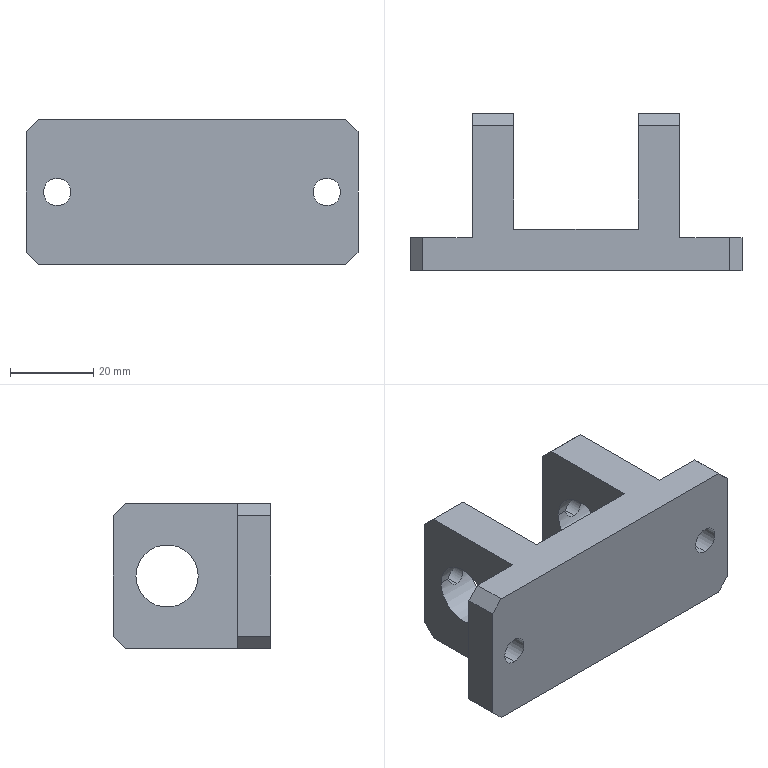Part | SolidWorks | features BaseBody 1 | 1 solid | 38 faces | box 80 x 38 x 35 mm | volume 36693 mm3 | plane 24 | cylinder 14 | commonest cylinder face diameters 5 x4 6.6 x4 15 x4 6 x2
STEP:
#1=CARTESIAN_POINT('',(20.,13.071,-2.5));
#2=VERTEX_POINT('',#1);
#3=CARTESIAN_POINT('',(17.5,13.5,0.));
#4=VERTEX_POINT('',#3);
#5=CARTESIAN_POINT('',(20.,13.071,-2.5));
#6=CARTESIAN_POINT('',(19.836,13.071,-2.5));
#7=CARTESIAN_POINT('',(19.671,13.077,-2.484));
#8=CARTESIAN_POINT('',(19.347,13.099,-2.419));
#9=CARTESIAN_POINT('',(19.191,13.116,-2.371));
#10=CARTESIAN_POINT('',(18.889,13.156,-2.246));
#11=CARTESIAN_POINT('',(18.743,13.181,-2.167));
#12=CARTESIAN_POINT('',(18.473,13.233,-1.986));
#13=CARTESIAN_POINT('',(18.348,13.261,-1.883));
#14=CARTESIAN_POINT('',(18.002,13.345,-1.537));
#15=CARTESIAN_POINT('',(17.818,13.399,-1.265));
#16=CARTESIAN_POINT('',(17.629,13.458,-0.8086));
#17=CARTESIAN_POINT('',(17.581,13.473,-0.6524));
#18=CARTESIAN_POINT('',(17.517,13.494,-0.3315));
#19=CARTESIAN_POINT('',(17.5,13.5,-0.1647));
#20=CARTESIAN_POINT('',(17.5,13.5,0.));
#21=B_SPLINE_CURVE_WITH_KNOTS('',3,(#5,#6,#7,#8,#9,#10,#11,#12,#13,#14,#15,#16,#17,#18,#19,#20),.UNSPECIFIED.,.F.,.F.,(4,2,2,2,2,2,2,4),(0.007873,0.008365,0.008856,0.009348,0.00984,0.01082,0.01132,0.01181),.UNSPECIFIED.);
#22=EDGE_CURVE('',#2,#4,#21,.T.);
#23=ORIENTED_EDGE('',*,*,#22,.F.);
#24=CARTESIAN_POINT('',(20.,19.,-2.5));
#25=VERTEX_POINT('',#24);
#26=CARTESIAN_POINT('',(20.,19.,-2.5));
#27=DIRECTION('',(0.,1.,0.));
#28=VECTOR('',#27,1000.);
#29=LINE('',#26,#28);
#30=EDGE_CURVE('',#2,#25,#29,.T.);
#31=ORIENTED_EDGE('',*,*,#30,.T.);
#32=CARTESIAN_POINT('',(20.,19.,2.5));
#33=VERTEX_POINT('',#32);
#34=CARTESIAN_POINT('',(20.,19.,0.));
#35=DIRECTION('',(0.,1.,0.));
#36=DIRECTION('',(0.,0.,1.));
#37=AXIS2_PLACEMENT_3D('',#34,#35,#36);
#38=CIRCLE('',#37,2.5);
#39=EDGE_CURVE('',#25,#33,#38,.T.);
#40=ORIENTED_EDGE('',*,*,#39,.T.);
#41=CARTESIAN_POINT('',(20.,13.071,2.5));
#42=VERTEX_POINT('',#41);
#43=CARTESIAN_POINT('',(20.,19.,2.5));
#44=DIRECTION('',(0.,1.,0.));
#45=VECTOR('',#44,1000.);
#46=LINE('',#43,#45);
#47=EDGE_CURVE('',#42,#33,#46,.T.);
#48=ORIENTED_EDGE('',*,*,#47,.F.);
#49=CARTESIAN_POINT('',(17.5,13.5,0.));
#50=CARTESIAN_POINT('',(17.5,13.5,0.1647));
#51=CARTESIAN_POINT('',(17.516,13.495,0.3279));
#52=CARTESIAN_POINT('',(17.581,13.473,0.6511));
#53=CARTESIAN_POINT('',(17.629,13.458,0.8102));
#54=CARTESIAN_POINT('',(17.817,13.399,1.262));
#55=CARTESIAN_POINT('',(18.003,13.344,1.539));
#56=CARTESIAN_POINT('',(18.347,13.261,1.882));
#57=CARTESIAN_POINT('',(18.474,13.233,1.987));
#58=CARTESIAN_POINT('',(18.745,13.18,2.168));
#59=CARTESIAN_POINT('',(18.888,13.156,2.245));
#60=CARTESIAN_POINT('',(19.19,13.116,2.371));
#61=CARTESIAN_POINT('',(19.349,13.099,2.419));
#62=CARTESIAN_POINT('',(19.67,13.077,2.484));
#63=CARTESIAN_POINT('',(19.834,13.071,2.5));
#64=CARTESIAN_POINT('',(20.,13.071,2.5));
#65=B_SPLINE_CURVE_WITH_KNOTS('',3,(#49,#50,#51,#52,#53,#54,#55,#56,#57,#58,#59,#60,#61,#62,#63,#64),.UNSPECIFIED.,.F.,.F.,(4,2,2,2,2,2,2,4),(0.01181,0.0123,0.01279,0.01378,0.01427,0.01476,0.01525,0.01574),.UNSPECIFIED.);
#66=EDGE_CURVE('',#4,#42,#65,.T.);
#67=ORIENTED_EDGE('',*,*,#66,.F.);
#68=EDGE_LOOP('',(#23,#31,#40,#48,#67));
#69=FACE_OUTER_BOUND('',#68,.T.);
#70=CARTESIAN_POINT('',(20.,19.,0.));
#71=DIRECTION('',(0.,1.,0.));
#72=DIRECTION('',(0.,0.,1.));
#73=AXIS2_PLACEMENT_3D('',#70,#71,#72);
#74=CYLINDRICAL_SURFACE('',#73,2.5);
#75=ADVANCED_FACE('',(#69),#74,.F.);
#76=CARTESIAN_POINT('',(-20.,13.071,-2.5));
#77=VERTEX_POINT('',#76);
#78=CARTESIAN_POINT('',(-22.5,13.5,0.));
#79=VERTEX_POINT('',#78);
#80=CARTESIAN_POINT('',(-20.,13.071,-2.5));
#81=CARTESIAN_POINT('',(-20.164,13.071,-2.5));
#82=CARTESIAN_POINT('',(-20.329,13.077,-2.484));
#83=CARTESIAN_POINT('',(-20.653,13.099,-2.419));
#84=CARTESIAN_POINT('',(-20.809,13.116,-2.371));
#85=CARTESIAN_POINT('',(-21.111,13.156,-2.246));
#86=CARTESIAN_POINT('',(-21.257,13.181,-2.167));
#87=CARTESIAN_POINT('',(-21.527,13.233,-1.986));
#88=CARTESIAN_POINT('',(-21.652,13.261,-1.883));
#89=CARTESIAN_POINT('',(-21.998,13.345,-1.537));
#90=CARTESIAN_POINT('',(-22.182,13.399,-1.265));
#91=CARTESIAN_POINT('',(-22.371,13.458,-0.8086));
#92=CARTESIAN_POINT('',(-22.419,13.473,-0.6524));
#93=CARTESIAN_POINT('',(-22.483,13.494,-0.3315));
#94=CARTESIAN_POINT('',(-22.5,13.5,-0.1647));
#95=CARTESIAN_POINT('',(-22.5,13.5,0.));
#96=B_SPLINE_CURVE_WITH_KNOTS('',3,(#80,#81,#82,#83,#84,#85,#86,#87,#88,#89,#90,#91,#92,#93,#94,#95),.UNSPECIFIED.,.F.,.F.,(4,2,2,2,2,2,2,4),(0.007873,0.008365,0.008856,0.009348,0.00984,0.01082,0.01132,0.01181),.UNSPECIFIED.);
#97=EDGE_CURVE('',#77,#79,#96,.T.);
#98=ORIENTED_EDGE('',*,*,#97,.F.);
#99=CARTESIAN_POINT('',(-20.,19.,-2.5));
#100=VERTEX_POINT('',#99);
#101=CARTESIAN_POINT('',(-20.,19.,-2.5));
#102=DIRECTION('',(0.,1.,0.));
#103=VECTOR('',#102,1000.);
#104=LINE('',#101,#103);
#105=EDGE_CURVE('',#77,#100,#104,.T.);
#106=ORIENTED_EDGE('',*,*,#105,.T.);
#107=CARTESIAN_POINT('',(-20.,19.,2.5));
#108=VERTEX_POINT('',#107);
#109=CARTESIAN_POINT('',(-20.,19.,0.));
#110=DIRECTION('',(0.,1.,0.));
#111=DIRECTION('',(0.,0.,1.));
#112=AXIS2_PLACEMENT_3D('',#109,#110,#111);
#113=CIRCLE('',#112,2.5);
#114=EDGE_CURVE('',#100,#108,#113,.T.);
#115=ORIENTED_EDGE('',*,*,#114,.T.);
#116=CARTESIAN_POINT('',(-20.,13.071,2.5));
#117=VERTEX_POINT('',#116);
#118=CARTESIAN_POINT('',(-20.,19.,2.5));
#119=DIRECTION('',(0.,1.,0.));
#120=VECTOR('',#119,1000.);
#121=LINE('',#118,#120);
#122=EDGE_CURVE('',#117,#108,#121,.T.);
#123=ORIENTED_EDGE('',*,*,#122,.F.);
#124=CARTESIAN_POINT('',(-22.5,13.5,0.));
#125=CARTESIAN_POINT('',(-22.5,13.5,0.1647));
#126=CARTESIAN_POINT('',(-22.484,13.495,0.3279));
#127=CARTESIAN_POINT('',(-22.419,13.473,0.6511));
#128=CARTESIAN_POINT('',(-22.371,13.458,0.8102));
#129=CARTESIAN_POINT('',(-22.183,13.399,1.262));
#130=CARTESIAN_POINT('',(-21.997,13.344,1.539));
#131=CARTESIAN_POINT('',(-21.653,13.261,1.882));
#132=CARTESIAN_POINT('',(-21.526,13.233,1.987));
#133=CARTESIAN_POINT('',(-21.255,13.18,2.168));
#134=CARTESIAN_POINT('',(-21.112,13.156,2.245));
#135=CARTESIAN_POINT('',(-20.81,13.116,2.371));
#136=CARTESIAN_POINT('',(-20.651,13.099,2.419));
#137=CARTESIAN_POINT('',(-20.33,13.077,2.484));
#138=CARTESIAN_POINT('',(-20.166,13.071,2.5));
#139=CARTESIAN_POINT('',(-20.,13.071,2.5));
#140=B_SPLINE_CURVE_WITH_KNOTS('',3,(#124,#125,#126,#127,#128,#129,#130,#131,#132,#133,#134,#135,#136,#137,#138,#139),.UNSPECIFIED.,.F.,.F.,(4,2,2,2,2,2,2,4),(0.01181,0.0123,0.01279,0.01378,0.01427,0.01476,0.01525,0.01574),.UNSPECIFIED.);
#141=EDGE_CURVE('',#79,#117,#140,.T.);
#142=ORIENTED_EDGE('',*,*,#141,.F.);
#143=EDGE_LOOP('',(#98,#106,#115,#123,#142));
#144=FACE_OUTER_BOUND('',#143,.T.);
#145=CARTESIAN_POINT('',(-20.,19.,0.));
#146=DIRECTION('',(0.,1.,0.));
#147=DIRECTION('',(0.,0.,1.));
#148=AXIS2_PLACEMENT_3D('',#145,#146,#147);
#149=CYLINDRICAL_SURFACE('',#148,2.5);
#150=ADVANCED_FACE('',(#144),#149,.F.);
#151=CARTESIAN_POINT('',(-32.5,-19.,-3.3));
#152=VERTEX_POINT('',#151);
#153=CARTESIAN_POINT('',(-32.5,-19.,3.3));
#154=VERTEX_POINT('',#153);
#155=CARTESIAN_POINT('',(-32.5,-19.,0.));
#156=DIRECTION('',(0.,1.,0.));
#157=DIRECTION('',(0.,0.,1.));
#158=AXIS2_PLACEMENT_3D('',#155,#156,#157);
#159=CIRCLE('',#158,3.3);
#160=EDGE_CURVE('',#152,#154,#159,.T.);
#161=ORIENTED_EDGE('',*,*,#160,.F.);
#162=CARTESIAN_POINT('',(-32.5,-11.,-3.3));
#163=VERTEX_POINT('',#162);
#164=CARTESIAN_POINT('',(-32.5,-11.,-3.3));
#165=DIRECTION('',(0.,1.,0.));
#166=VECTOR('',#165,1000.);
#167=LINE('',#164,#166);
#168=EDGE_CURVE('',#152,#163,#167,.T.);
#169=ORIENTED_EDGE('',*,*,#168,.T.);
#170=CARTESIAN_POINT('',(-32.5,-11.,3.3));
#171=VERTEX_POINT('',#170);
#172=CARTESIAN_POINT('',(-32.5,-11.,0.));
#173=DIRECTION('',(0.,1.,0.));
#174=DIRECTION('',(0.,0.,1.));
#175=AXIS2_PLACEMENT_3D('',#172,#173,#174);
#176=CIRCLE('',#175,3.3);
#177=EDGE_CURVE('',#163,#171,#176,.T.);
#178=ORIENTED_EDGE('',*,*,#177,.T.);
#179=CARTESIAN_POINT('',(-32.5,-11.,3.3));
#180=DIRECTION('',(0.,1.,0.));
#181=VECTOR('',#180,1000.);
#182=LINE('',#179,#181);
#183=EDGE_CURVE('',#154,#171,#182,.T.);
#184=ORIENTED_EDGE('',*,*,#183,.F.);
#185=EDGE_LOOP('',(#161,#169,#178,#184));
#186=FACE_OUTER_BOUND('',#185,.T.);
#187=CARTESIAN_POINT('',(-32.5,-11.,0.));
#188=DIRECTION('',(0.,1.,0.));
#189=DIRECTION('',(0.,0.,1.));
#190=AXIS2_PLACEMENT_3D('',#187,#188,#189);
#191=CYLINDRICAL_SURFACE('',#190,3.3);
#192=ADVANCED_FACE('',(#186),#191,.F.);
#193=CARTESIAN_POINT('',(32.5,-19.,-3.3));
#194=VERTEX_POINT('',#193);
#195=CARTESIAN_POINT('',(32.5,-19.,3.3));
#196=VERTEX_POINT('',#195);
#197=CARTESIAN_POINT('',(32.5,-19.,0.));
#198=DIRECTION('',(0.,1.,0.));
#199=DIRECTION('',(0.,0.,1.));
#200=AXIS2_PLACEMENT_3D('',#197,#198,#199);
#201=CIRCLE('',#200,3.3);
#202=EDGE_CURVE('',#194,#196,#201,.T.);
#203=ORIENTED_EDGE('',*,*,#202,.F.);
#204=CARTESIAN_POINT('',(32.5,-11.,-3.3));
#205=VERTEX_POINT('',#204);
#206=CARTESIAN_POINT('',(32.5,-11.,-3.3));
#207=DIRECTION('',(0.,1.,0.));
#208=VECTOR('',#207,1000.);
#209=LINE('',#206,#208);
#210=EDGE_CURVE('',#194,#205,#209,.T.);
#211=ORIENTED_EDGE('',*,*,#210,.T.);
#212=CARTESIAN_POINT('',(32.5,-11.,3.3));
#213=VERTEX_POINT('',#212);
#214=CARTESIAN_POINT('',(32.5,-11.,0.));
#215=DIRECTION('',(0.,1.,0.));
#216=DIRECTION('',(0.,0.,1.));
#217=AXIS2_PLACEMENT_3D('',#214,#215,#216);
#218=CIRCLE('',#217,3.3);
#219=EDGE_CURVE('',#205,#213,#218,.T.);
#220=ORIENTED_EDGE('',*,*,#219,.T.);
#221=CARTESIAN_POINT('',(32.5,-11.,3.3));
#222=DIRECTION('',(0.,1.,0.));
#223=VECTOR('',#222,1000.);
#224=LINE('',#221,#223);
#225=EDGE_CURVE('',#196,#213,#224,.T.);
#226=ORIENTED_EDGE('',*,*,#225,.F.);
#227=EDGE_LOOP('',(#203,#211,#220,#226));
#228=FACE_OUTER_BOUND('',#227,.T.);
#229=CARTESIAN_POINT('',(32.5,-11.,0.));
#230=DIRECTION('',(0.,1.,0.));
#231=DIRECTION('',(0.,0.,1.));
#232=AXIS2_PLACEMENT_3D('',#229,#230,#231);
#233=CYLINDRICAL_SURFACE('',#232,3.3);
#234=ADVANCED_FACE('',(#228),#233,.F.);
#235=CARTESIAN_POINT('',(25.,13.5,0.));
#236=VERTEX_POINT('',#235);
#237=CARTESIAN_POINT('',(25.,-1.5,0.));
#238=VERTEX_POINT('',#237);
#239=CARTESIAN_POINT('',(25.,6.,0.));
#240=DIRECTION('',(-1.,0.,0.));
#241=DIRECTION('',(0.,-1.,0.));
#242=AXIS2_PLACEMENT_3D('',#239,#240,#241);
#243=CIRCLE('',#242,7.5);
#244=EDGE_CURVE('',#236,#238,#243,.T.);
#245=ORIENTED_EDGE('',*,*,#244,.F.);
#246=CARTESIAN_POINT('',(22.5,13.5,0.));
#247=VERTEX_POINT('',#246);
#248=CARTESIAN_POINT('',(40.,13.5,0.));
#249=DIRECTION('',(-1.,0.,0.));
#250=VECTOR('',#249,1000.);
#251=LINE('',#248,#250);
#252=EDGE_CURVE('',#236,#247,#251,.T.);
#253=ORIENTED_EDGE('',*,*,#252,.T.);
#254=CARTESIAN_POINT('',(22.5,13.5,0.));
#255=CARTESIAN_POINT('',(22.5,13.5,-0.1644));
#256=CARTESIAN_POINT('',(22.483,13.494,-0.3313));
#257=CARTESIAN_POINT('',(22.419,13.473,-0.6529));
#258=CARTESIAN_POINT('',(22.371,13.458,-0.8094));
#259=CARTESIAN_POINT('',(22.244,13.418,-1.114));
#260=CARTESIAN_POINT('',(22.167,13.395,-1.258));
#261=CARTESIAN_POINT('',(21.986,13.344,-1.527));
#262=CARTESIAN_POINT('',(21.881,13.316,-1.654));
#263=CARTESIAN_POINT('',(21.651,13.26,-1.884));
#264=CARTESIAN_POINT('',(21.526,13.233,-1.987));
#265=CARTESIAN_POINT('',(21.256,13.181,-2.168));
#266=CARTESIAN_POINT('',(21.11,13.156,-2.246));
#267=CARTESIAN_POINT('',(20.809,13.116,-2.371));
#268=CARTESIAN_POINT('',(20.653,13.099,-2.419));
#269=CARTESIAN_POINT('',(20.33,13.077,-2.484));
#270=CARTESIAN_POINT('',(20.164,13.071,-2.5));
#271=CARTESIAN_POINT('',(20.,13.071,-2.5));
#272=B_SPLINE_CURVE_WITH_KNOTS('',3,(#254,#255,#256,#257,#258,#259,#260,#261,#262,#263,#264,#265,#266,#267,#268,#269,#270,#271),.UNSPECIFIED.,.F.,.F.,(4,2,2,2,2,2,2,2,4),(0.003937,0.004429,0.004921,0.005413,0.005905,0.006397,0.006889,0.007381,0.007873),.UNSPECIFIED.);
#273=EDGE_CURVE('',#247,#2,#272,.T.);
#274=ORIENTED_EDGE('',*,*,#273,.T.);
#275=ORIENTED_EDGE('',*,*,#22,.T.);
#276=CARTESIAN_POINT('',(15.,13.5,0.));
#277=VERTEX_POINT('',#276);
#278=CARTESIAN_POINT('',(40.,13.5,0.));
#279=DIRECTION('',(-1.,0.,0.));
#280=VECTOR('',#279,1000.);
#281=LINE('',#278,#280);
#282=EDGE_CURVE('',#4,#277,#281,.T.);
#283=ORIENTED_EDGE('',*,*,#282,.T.);
#284=CARTESIAN_POINT('',(15.,-1.5,0.));
#285=VERTEX_POINT('',#284);
#286=CARTESIAN_POINT('',(15.,6.,0.));
#287=DIRECTION('',(-1.,0.,0.));
#288=DIRECTION('',(0.,1.,0.));
#289=AXIS2_PLACEMENT_3D('',#286,#287,#288);
#290=CIRCLE('',#289,7.5);
#291=EDGE_CURVE('',#277,#285,#290,.T.);
#292=ORIENTED_EDGE('',*,*,#291,.T.);
#293=CARTESIAN_POINT('',(40.,-1.5,0.));
#294=DIRECTION('',(-1.,0.,0.));
#295=VECTOR('',#294,1000.);
#296=LINE('',#293,#295);
#297=EDGE_CURVE('',#238,#285,#296,.T.);
#298=ORIENTED_EDGE('',*,*,#297,.F.);
#299=EDGE_LOOP('',(#245,#253,#274,#275,#283,#292,#298));
#300=FACE_OUTER_BOUND('',#299,.T.);
#301=CARTESIAN_POINT('',(40.,6.,0.));
#302=DIRECTION('',(-1.,0.,0.));
#303=DIRECTION('',(0.,-1.,0.));
#304=AXIS2_PLACEMENT_3D('',#301,#302,#303);
#305=CYLINDRICAL_SURFACE('',#304,7.5);
#306=ADVANCED_FACE('',(#300),#305,.F.);
#307=CARTESIAN_POINT('',(-15.,-1.5,0.));
#308=VERTEX_POINT('',#307);
#309=CARTESIAN_POINT('',(-15.,13.5,0.));
#310=VERTEX_POINT('',#309);
#311=CARTESIAN_POINT('',(-15.,6.,0.));
#312=DIRECTION('',(1.,0.,0.));
#313=DIRECTION('',(0.,-1.,0.));
#314=AXIS2_PLACEMENT_3D('',#311,#312,#313);
#315=CIRCLE('',#314,7.5);
#316=EDGE_CURVE('',#308,#310,#315,.T.);
#317=ORIENTED_EDGE('',*,*,#316,.T.);
#318=CARTESIAN_POINT('',(-17.5,13.5,0.));
#319=VERTEX_POINT('',#318);
#320=CARTESIAN_POINT('',(40.,13.5,0.));
#321=DIRECTION('',(-1.,0.,0.));
#322=VECTOR('',#321,1000.);
#323=LINE('',#320,#322);
#324=EDGE_CURVE('',#310,#319,#323,.T.);
#325=ORIENTED_EDGE('',*,*,#324,.T.);
#326=CARTESIAN_POINT('',(-17.5,13.5,0.));
#327=CARTESIAN_POINT('',(-17.5,13.5,-0.1644));
#328=CARTESIAN_POINT('',(-17.517,13.494,-0.3313));
#329=CARTESIAN_POINT('',(-17.581,13.473,-0.6529));
#330=CARTESIAN_POINT('',(-17.629,13.458,-0.8094));
#331=CARTESIAN_POINT('',(-17.756,13.418,-1.114));
#332=CARTESIAN_POINT('',(-17.833,13.395,-1.258));
#333=CARTESIAN_POINT('',(-18.014,13.344,-1.527));
#334=CARTESIAN_POINT('',(-18.119,13.316,-1.654));
#335=CARTESIAN_POINT('',(-18.349,13.26,-1.884));
#336=CARTESIAN_POINT('',(-18.474,13.233,-1.987));
#337=CARTESIAN_POINT('',(-18.744,13.181,-2.168));
#338=CARTESIAN_POINT('',(-18.89,13.156,-2.246));
#339=CARTESIAN_POINT('',(-19.191,13.116,-2.371));
#340=CARTESIAN_POINT('',(-19.347,13.099,-2.419));
#341=CARTESIAN_POINT('',(-19.67,13.077,-2.484));
#342=CARTESIAN_POINT('',(-19.836,13.071,-2.5));
#343=CARTESIAN_POINT('',(-20.,13.071,-2.5));
#344=B_SPLINE_CURVE_WITH_KNOTS('',3,(#326,#327,#328,#329,#330,#331,#332,#333,#334,#335,#336,#337,#338,#339,#340,#341,#342,#343),.UNSPECIFIED.,.F.,.F.,(4,2,2,2,2,2,2,2,4),(0.003937,0.004429,0.004921,0.005413,0.005905,0.006397,0.006889,0.007381,0.007873),.UNSPECIFIED.);
#345=EDGE_CURVE('',#319,#77,#344,.T.);
#346=ORIENTED_EDGE('',*,*,#345,.T.);
#347=ORIENTED_EDGE('',*,*,#97,.T.);
#348=CARTESIAN_POINT('',(-25.,13.5,0.));
#349=VERTEX_POINT('',#348);
#350=CARTESIAN_POINT('',(40.,13.5,0.));
#351=DIRECTION('',(-1.,0.,0.));
#352=VECTOR('',#351,1000.);
#353=LINE('',#350,#352);
#354=EDGE_CURVE('',#79,#349,#353,.T.);
#355=ORIENTED_EDGE('',*,*,#354,.T.);
#356=CARTESIAN_POINT('',(-25.,-1.5,0.));
#357=VERTEX_POINT('',#356);
#358=CARTESIAN_POINT('',(-25.,6.,0.));
#359=DIRECTION('',(-1.,0.,0.));
#360=DIRECTION('',(0.,-1.,0.));
#361=AXIS2_PLACEMENT_3D('',#358,#359,#360);
#362=CIRCLE('',#361,7.5);
#363=EDGE_CURVE('',#349,#357,#362,.T.);
#364=ORIENTED_EDGE('',*,*,#363,.T.);
#365=CARTESIAN_POINT('',(40.,-1.5,0.));
#366=DIRECTION('',(-1.,0.,0.));
#367=VECTOR('',#366,1000.);
#368=LINE('',#365,#367);
#369=EDGE_CURVE('',#308,#357,#368,.T.);
#370=ORIENTED_EDGE('',*,*,#369,.F.);
#371=EDGE_LOOP('',(#317,#325,#346,#347,#355,#364,#370));
#372=FACE_OUTER_BOUND('',#371,.T.);
#373=CARTESIAN_POINT('',(40.,6.,0.));
#374=DIRECTION('',(-1.,0.,0.));
#375=DIRECTION('',(0.,-1.,0.));
#376=AXIS2_PLACEMENT_3D('',#373,#374,#375);
#377=CYLINDRICAL_SURFACE('',#376,7.5);
#378=ADVANCED_FACE('',(#372),#377,.F.);
#379=CARTESIAN_POINT('',(-20.,19.,0.));
#380=DIRECTION('',(0.,1.,0.));
#381=DIRECTION('',(0.,0.,1.));
#382=AXIS2_PLACEMENT_3D('',#379,#380,#381);
#383=CIRCLE('',#382,2.5);
#384=EDGE_CURVE('',#108,#100,#383,.T.);
#385=ORIENTED_EDGE('',*,*,#384,.F.);
#386=ORIENTED_EDGE('',*,*,#114,.F.);
#387=EDGE_LOOP('',(#385,#386));
#388=FACE_BOUND('',#387,.T.);
#389=CARTESIAN_POINT('',(-25.,19.,-14.5));
#390=VERTEX_POINT('',#389);
#391=CARTESIAN_POINT('',(-25.,19.,14.5));
#392=VERTEX_POINT('',#391);
#393=CARTESIAN_POINT('',(-25.,19.,-17.5));
#394=DIRECTION('',(0.,0.,1.));
#395=VECTOR('',#394,1000.);
#396=LINE('',#393,#395);
#397=EDGE_CURVE('',#390,#392,#396,.T.);
#398=ORIENTED_EDGE('',*,*,#397,.T.);
#399=CARTESIAN_POINT('',(-15.,19.,14.5));
#400=VERTEX_POINT('',#399);
#401=CARTESIAN_POINT('',(40.,19.,14.5));
#402=DIRECTION('',(1.,0.,0.));
#403=VECTOR('',#402,1000.);
#404=LINE('',#401,#403);
#405=EDGE_CURVE('',#392,#400,#404,.T.);
#406=ORIENTED_EDGE('',*,*,#405,.T.);
#407=CARTESIAN_POINT('',(-15.,19.,-14.5));
#408=VERTEX_POINT('',#407);
#409=CARTESIAN_POINT('',(-15.,19.,-17.5));
#410=DIRECTION('',(0.,0.,1.));
#411=VECTOR('',#410,1000.);
#412=LINE('',#409,#411);
#413=EDGE_CURVE('',#408,#400,#412,.T.);
#414=ORIENTED_EDGE('',*,*,#413,.F.);
#415=CARTESIAN_POINT('',(-25.,19.,-14.5));
#416=DIRECTION('',(-1.,0.,0.));
#417=VECTOR('',#416,1000.);
#418=LINE('',#415,#417);
#419=EDGE_CURVE('',#408,#390,#418,.T.);
#420=ORIENTED_EDGE('',*,*,#419,.T.);
#421=EDGE_LOOP('',(#398,#406,#414,#420));
#422=FACE_OUTER_BOUND('',#421,.T.);
#423=CARTESIAN_POINT('',(40.,19.,17.5));
#424=DIRECTION('',(0.,-1.,0.));
#425=DIRECTION('',(1.,0.,0.));
#426=AXIS2_PLACEMENT_3D('',#423,#424,#425);
#427=PLANE('',#426);
#428=ADVANCED_FACE('',(#388,#422),#427,.F.);
#429=ORIENTED_EDGE('',*,*,#324,.F.);
#430=CARTESIAN_POINT('',(-15.,6.,0.));
#431=DIRECTION('',(1.,0.,0.));
#432=DIRECTION('',(0.,-1.,0.));
#433=AXIS2_PLACEMENT_3D('',#430,#431,#432);
#434=CIRCLE('',#433,7.5);
#435=EDGE_CURVE('',#310,#308,#434,.T.);
#436=ORIENTED_EDGE('',*,*,#435,.T.);
#437=ORIENTED_EDGE('',*,*,#369,.T.);
#438=CARTESIAN_POINT('',(-25.,6.,0.));
#439=DIRECTION('',(-1.,0.,0.));
#440=DIRECTION('',(0.,-1.,0.));
#441=AXIS2_PLACEMENT_3D('',#438,#439,#440);
#442=CIRCLE('',#441,7.5);
#443=EDGE_CURVE('',#357,#349,#442,.T.);
#444=ORIENTED_EDGE('',*,*,#443,.T.);
#445=ORIENTED_EDGE('',*,*,#354,.F.);
#446=ORIENTED_EDGE('',*,*,#141,.T.);
#447=CARTESIAN_POINT('',(-20.,13.071,2.5));
#448=CARTESIAN_POINT('',(-19.833,13.071,2.5));
#449=CARTESIAN_POINT('',(-19.67,13.077,2.484));
#450=CARTESIAN_POINT('',(-19.349,13.099,2.419));
#451=CARTESIAN_POINT('',(-19.189,13.116,2.371));
#452=CARTESIAN_POINT('',(-18.887,13.157,2.245));
#453=CARTESIAN_POINT('',(-18.744,13.181,2.168));
#454=CARTESIAN_POINT('',(-18.473,13.233,1.986));
#455=CARTESIAN_POINT('',(-18.346,13.261,1.882));
#456=CARTESIAN_POINT('',(-18.003,13.344,1.538));
#457=CARTESIAN_POINT('',(-17.817,13.399,1.261));
#458=CARTESIAN_POINT('',(-17.629,13.458,0.81));
#459=CARTESIAN_POINT('',(-17.581,13.473,0.6511));
#460=CARTESIAN_POINT('',(-17.516,13.495,0.3276));
#461=CARTESIAN_POINT('',(-17.5,13.5,0.1645));
#462=CARTESIAN_POINT('',(-17.5,13.5,0.));
#463=B_SPLINE_CURVE_WITH_KNOTS('',3,(#447,#448,#449,#450,#451,#452,#453,#454,#455,#456,#457,#458,#459,#460,#461,#462),.UNSPECIFIED.,.F.,.F.,(4,2,2,2,2,2,2,4),(0.,0.0004922,0.0009844,0.001477,0.001969,0.002953,0.003445,0.003937),.UNSPECIFIED.);
#464=EDGE_CURVE('',#117,#319,#463,.T.);
#465=ORIENTED_EDGE('',*,*,#464,.T.);
#466=EDGE_LOOP('',(#429,#436,#437,#444,#445,#446,#465));
#467=FACE_OUTER_BOUND('',#466,.T.);
#468=CARTESIAN_POINT('',(40.,6.,0.));
#469=DIRECTION('',(-1.,0.,0.));
#470=DIRECTION('',(0.,-1.,0.));
#471=AXIS2_PLACEMENT_3D('',#468,#469,#470);
#472=CYLINDRICAL_SURFACE('',#471,7.5);
#473=ADVANCED_FACE('',(#467),#472,.F.);
#474=CARTESIAN_POINT('',(-40.,-19.,14.5));
#475=VERTEX_POINT('',#474);
#476=CARTESIAN_POINT('',(-40.,-19.,-14.5));
#477=VERTEX_POINT('',#476);
#478=CARTESIAN_POINT('',(-40.,-19.,17.5));
#479=DIRECTION('',(0.,0.,-1.));
#480=VECTOR('',#479,1000.);
#481=LINE('',#478,#480);
#482=EDGE_CURVE('',#475,#477,#481,.T.);
#483=ORIENTED_EDGE('',*,*,#482,.F.);
#484=CARTESIAN_POINT('',(-40.,-11.,14.5));
#485=VERTEX_POINT('',#484);
#486=CARTESIAN_POINT('',(-40.,19.,14.5));
#487=DIRECTION('',(0.,1.,0.));
#488=VECTOR('',#487,1000.);
#489=LINE('',#486,#488);
#490=EDGE_CURVE('',#475,#485,#489,.T.);
#491=ORIENTED_EDGE('',*,*,#490,.T.);
#492=CARTESIAN_POINT('',(-40.,-11.,-14.5));
#493=VERTEX_POINT('',#492);
#494=CARTESIAN_POINT('',(-40.,-11.,-17.5));
#495=DIRECTION('',(0.,0.,1.));
#496=VECTOR('',#495,1000.);
#497=LINE('',#494,#496);
#498=EDGE_CURVE('',#493,#485,#497,.T.);
#499=ORIENTED_EDGE('',*,*,#498,.F.);
#500=CARTESIAN_POINT('',(-40.,-19.,-14.5));
#501=DIRECTION('',(0.,-1.,0.));
#502=VECTOR('',#501,1000.);
#503=LINE('',#500,#502);
#504=EDGE_CURVE('',#493,#477,#503,.T.);
#505=ORIENTED_EDGE('',*,*,#504,.T.);
#506=EDGE_LOOP('',(#483,#491,#499,#505));
#507=FACE_OUTER_BOUND('',#506,.T.);
#508=CARTESIAN_POINT('',(-40.,19.,17.5));
#509=DIRECTION('',(1.,0.,0.));
#510=DIRECTION('',(0.,1.,0.));
#511=AXIS2_PLACEMENT_3D('',#508,#509,#510);
#512=PLANE('',#511);
#513=ADVANCED_FACE('',(#507),#512,.F.);
#514=CARTESIAN_POINT('',(-32.5,-19.,0.));
#515=DIRECTION('',(0.,1.,0.));
#516=DIRECTION('',(0.,0.,1.));
#517=AXIS2_PLACEMENT_3D('',#514,#515,#516);
#518=CIRCLE('',#517,3.3);
#519=EDGE_CURVE('',#154,#152,#518,.T.);
#520=ORIENTED_EDGE('',*,*,#519,.T.);
#521=ORIENTED_EDGE('',*,*,#160,.T.);
#522=EDGE_LOOP('',(#520,#521));
#523=FACE_BOUND('',#522,.T.);
#524=CARTESIAN_POINT('',(32.5,-19.,0.));
#525=DIRECTION('',(0.,1.,0.));
#526=DIRECTION('',(0.,0.,1.));
#527=AXIS2_PLACEMENT_3D('',#524,#525,#526);
#528=CIRCLE('',#527,3.3);
#529=EDGE_CURVE('',#196,#194,#528,.T.);
#530=ORIENTED_EDGE('',*,*,#529,.T.);
#531=ORIENTED_EDGE('',*,*,#202,.T.);
#532=EDGE_LOOP('',(#530,#531));
#533=FACE_BOUND('',#532,.T.);
#534=CARTESIAN_POINT('',(-37.,-19.,-17.5));
#535=VERTEX_POINT('',#534);
#536=CARTESIAN_POINT('',(37.,-19.,-17.5));
#537=VERTEX_POINT('',#536);
#538=CARTESIAN_POINT('',(40.,-19.,-17.5));
#539=DIRECTION('',(1.,0.,0.));
#540=VECTOR('',#539,1000.);
#541=LINE('',#538,#540);
#542=EDGE_CURVE('',#535,#537,#541,.T.);
#543=ORIENTED_EDGE('',*,*,#542,.T.);
#544=CARTESIAN_POINT('',(40.,-19.,-14.5));
#545=VERTEX_POINT('',#544);
#546=CARTESIAN_POINT('',(40.,-19.,-14.5));
#547=DIRECTION('',(0.7071,0.,0.7071));
#548=VECTOR('',#547,1000.);
#549=LINE('',#546,#548);
#550=EDGE_CURVE('',#537,#545,#549,.T.);
#551=ORIENTED_EDGE('',*,*,#550,.T.);
#552=CARTESIAN_POINT('',(40.,-19.,14.5));
#553=VERTEX_POINT('',#552);
#554=CARTESIAN_POINT('',(40.,-19.,17.5));
#555=DIRECTION('',(0.,0.,-1.));
#556=VECTOR('',#555,1000.);
#557=LINE('',#554,#556);
#558=EDGE_CURVE('',#553,#545,#557,.T.);
#559=ORIENTED_EDGE('',*,*,#558,.F.);
#560=CARTESIAN_POINT('',(37.,-19.,17.5));
#561=VERTEX_POINT('',#560);
#562=CARTESIAN_POINT('',(37.,-19.,17.5));
#563=DIRECTION('',(-0.7071,0.,0.7071));
#564=VECTOR('',#563,1000.);
#565=LINE('',#562,#564);
#566=EDGE_CURVE('',#553,#561,#565,.T.);
#567=ORIENTED_EDGE('',*,*,#566,.T.);
#568=CARTESIAN_POINT('',(-37.,-19.,17.5));
#569=VERTEX_POINT('',#568);
#570=CARTESIAN_POINT('',(40.,-19.,17.5));
#571=DIRECTION('',(1.,0.,0.));
#572=VECTOR('',#571,1000.);
#573=LINE('',#570,#572);
#574=EDGE_CURVE('',#569,#561,#573,.T.);
#575=ORIENTED_EDGE('',*,*,#574,.F.);
#576=CARTESIAN_POINT('',(-37.,-19.,17.5));
#577=DIRECTION('',(-0.7071,0.,-0.7071));
#578=VECTOR('',#577,1000.);
#579=LINE('',#576,#578);
#580=EDGE_CURVE('',#569,#475,#579,.T.);
#581=ORIENTED_EDGE('',*,*,#580,.T.);
#582=ORIENTED_EDGE('',*,*,#482,.T.);
#583=CARTESIAN_POINT('',(-40.,-19.,-14.5));
#584=DIRECTION('',(0.7071,0.,-0.7071));
#585=VECTOR('',#584,1000.);
#586=LINE('',#583,#585);
#587=EDGE_CURVE('',#477,#535,#586,.T.);
#588=ORIENTED_EDGE('',*,*,#587,.T.);
#589=EDGE_LOOP('',(#543,#551,#559,#567,#575,#581,#582,#588));
#590=FACE_OUTER_BOUND('',#589,.T.);
#591=CARTESIAN_POINT('',(40.,-19.,17.5));
#592=DIRECTION('',(0.,1.,0.));
#593=DIRECTION('',(-1.,0.,0.));
#594=AXIS2_PLACEMENT_3D('',#591,#592,#593);
#595=PLANE('',#594);
#596=ADVANCED_FACE('',(#523,#533,#590),#595,.F.);
#597=ORIENTED_EDGE('',*,*,#558,.T.);
#598=CARTESIAN_POINT('',(40.,-11.,-14.5));
#599=VERTEX_POINT('',#598);
#600=CARTESIAN_POINT('',(40.,-11.,-14.5));
#601=DIRECTION('',(0.,1.,0.));
#602=VECTOR('',#601,1000.);
#603=LINE('',#600,#602);
#604=EDGE_CURVE('',#545,#599,#603,.T.);
#605=ORIENTED_EDGE('',*,*,#604,.T.);
#606=CARTESIAN_POINT('',(40.,-11.,14.5));
#607=VERTEX_POINT('',#606);
#608=CARTESIAN_POINT('',(40.,-11.,-17.5));
#609=DIRECTION('',(0.,0.,1.));
#610=VECTOR('',#609,1000.);
#611=LINE('',#608,#610);
#612=EDGE_CURVE('',#599,#607,#611,.T.);
#613=ORIENTED_EDGE('',*,*,#612,.T.);
#614=CARTESIAN_POINT('',(40.,19.,14.5));
#615=DIRECTION('',(0.,-1.,0.));
#616=VECTOR('',#615,1000.);
#617=LINE('',#614,#616);
#618=EDGE_CURVE('',#607,#553,#617,.T.);
#619=ORIENTED_EDGE('',*,*,#618,.T.);
#620=EDGE_LOOP('',(#597,#605,#613,#619));
#621=FACE_OUTER_BOUND('',#620,.T.);
#622=CARTESIAN_POINT('',(40.,19.,17.5));
#623=DIRECTION('',(-1.,0.,0.));
#624=DIRECTION('',(0.,0.,1.));
#625=AXIS2_PLACEMENT_3D('',#622,#623,#624);
#626=PLANE('',#625);
#627=ADVANCED_FACE('',(#621),#626,.F.);
#628=CARTESIAN_POINT('',(20.,19.,0.));
#629=DIRECTION('',(0.,1.,0.));
#630=DIRECTION('',(0.,0.,1.));
#631=AXIS2_PLACEMENT_3D('',#628,#629,#630);
#632=CIRCLE('',#631,2.5);
#633=EDGE_CURVE('',#33,#25,#632,.T.);
#634=ORIENTED_EDGE('',*,*,#633,.F.);
#635=ORIENTED_EDGE('',*,*,#39,.F.);
#636=EDGE_LOOP('',(#634,#635));
#637=FACE_BOUND('',#636,.T.);
#638=CARTESIAN_POINT('',(15.,19.,-14.5));
#639=VERTEX_POINT('',#638);
#640=CARTESIAN_POINT('',(15.,19.,14.5));
#641=VERTEX_POINT('',#640);
#642=CARTESIAN_POINT('',(15.,19.,-17.5));
#643=DIRECTION('',(0.,0.,1.));
#644=VECTOR('',#643,1000.);
#645=LINE('',#642,#644);
#646=EDGE_CURVE('',#639,#641,#645,.T.);
#647=ORIENTED_EDGE('',*,*,#646,.T.);
#648=CARTESIAN_POINT('',(25.,19.,14.5));
#649=VERTEX_POINT('',#648);
#650=CARTESIAN_POINT('',(40.,19.,14.5));
#651=DIRECTION('',(1.,0.,0.));
#652=VECTOR('',#651,1000.);
#653=LINE('',#650,#652);
#654=EDGE_CURVE('',#641,#649,#653,.T.);
#655=ORIENTED_EDGE('',*,*,#654,.T.);
#656=CARTESIAN_POINT('',(25.,19.,-14.5));
#657=VERTEX_POINT('',#656);
#658=CARTESIAN_POINT('',(25.,19.,-17.5));
#659=DIRECTION('',(0.,0.,1.));
#660=VECTOR('',#659,1000.);
#661=LINE('',#658,#660);
#662=EDGE_CURVE('',#657,#649,#661,.T.);
#663=ORIENTED_EDGE('',*,*,#662,.F.);
#664=CARTESIAN_POINT('',(15.,19.,-14.5));
#665=DIRECTION('',(-1.,0.,0.));
#666=VECTOR('',#665,1000.);
#667=LINE('',#664,#666);
#668=EDGE_CURVE('',#657,#639,#667,.T.);
#669=ORIENTED_EDGE('',*,*,#668,.T.);
#670=EDGE_LOOP('',(#647,#655,#663,#669));
#671=FACE_OUTER_BOUND('',#670,.T.);
#672=CARTESIAN_POINT('',(40.,19.,17.5));
#673=DIRECTION('',(0.,-1.,0.));
#674=DIRECTION('',(1.,0.,0.));
#675=AXIS2_PLACEMENT_3D('',#672,#673,#674);
#676=PLANE('',#675);
#677=ADVANCED_FACE('',(#637,#671),#676,.F.);
#678=ORIENTED_EDGE('',*,*,#574,.T.);
#679=CARTESIAN_POINT('',(37.,-11.,17.5));
#680=VERTEX_POINT('',#679);
#681=CARTESIAN_POINT('',(37.,-19.,17.5));
#682=DIRECTION('',(0.,1.,0.));
#683=VECTOR('',#682,1000.);
#684=LINE('',#681,#683);
#685=EDGE_CURVE('',#561,#680,#684,.T.);
#686=ORIENTED_EDGE('',*,*,#685,.T.);
#687=CARTESIAN_POINT('',(25.,-11.,17.5));
#688=VERTEX_POINT('',#687);
#689=CARTESIAN_POINT('',(40.,-11.,17.5));
#690=DIRECTION('',(1.,0.,0.));
#691=VECTOR('',#690,1000.);
#692=LINE('',#689,#691);
#693=EDGE_CURVE('',#688,#680,#692,.T.);
#694=ORIENTED_EDGE('',*,*,#693,.F.);
#695=CARTESIAN_POINT('',(25.,16.,17.5));
#696=VERTEX_POINT('',#695);
#697=CARTESIAN_POINT('',(25.,19.,17.5));
#698=DIRECTION('',(0.,-1.,0.));
#699=VECTOR('',#698,1000.);
#700=LINE('',#697,#699);
#701=EDGE_CURVE('',#696,#688,#700,.T.);
#702=ORIENTED_EDGE('',*,*,#701,.F.);
#703=CARTESIAN_POINT('',(15.,16.,17.5));
#704=VERTEX_POINT('',#703);
#705=CARTESIAN_POINT('',(-40.,16.,17.5));
#706=DIRECTION('',(-1.,0.,0.));
#707=VECTOR('',#706,1000.);
#708=LINE('',#705,#707);
#709=EDGE_CURVE('',#696,#704,#708,.T.);
#710=ORIENTED_EDGE('',*,*,#709,.T.);
#711=CARTESIAN_POINT('',(15.,-9.,17.5));
#712=VERTEX_POINT('',#711);
#713=CARTESIAN_POINT('',(15.,19.,17.5));
#714=DIRECTION('',(0.,1.,0.));
#715=VECTOR('',#714,1000.);
#716=LINE('',#713,#715);
#717=EDGE_CURVE('',#712,#704,#716,.T.);
#718=ORIENTED_EDGE('',*,*,#717,.F.);
#719=CARTESIAN_POINT('',(-15.,-9.,17.5));
#720=VERTEX_POINT('',#719);
#721=CARTESIAN_POINT('',(-15.,-9.,17.5));
#722=DIRECTION('',(1.,0.,0.));
#723=VECTOR('',#722,1000.);
#724=LINE('',#721,#723);
#725=EDGE_CURVE('',#720,#712,#724,.T.);
#726=ORIENTED_EDGE('',*,*,#725,.F.);
#727=CARTESIAN_POINT('',(-15.,16.,17.5));
#728=VERTEX_POINT('',#727);
#729=CARTESIAN_POINT('',(-15.,19.,17.5));
#730=DIRECTION('',(0.,-1.,0.));
#731=VECTOR('',#730,1000.);
#732=LINE('',#729,#731);
#733=EDGE_CURVE('',#728,#720,#732,.T.);
#734=ORIENTED_EDGE('',*,*,#733,.F.);
#735=CARTESIAN_POINT('',(-25.,16.,17.5));
#736=VERTEX_POINT('',#735);
#737=CARTESIAN_POINT('',(-40.,16.,17.5));
#738=DIRECTION('',(-1.,0.,0.));
#739=VECTOR('',#738,1000.);
#740=LINE('',#737,#739);
#741=EDGE_CURVE('',#728,#736,#740,.T.);
#742=ORIENTED_EDGE('',*,*,#741,.T.);
#743=CARTESIAN_POINT('',(-25.,-11.,17.5));
#744=VERTEX_POINT('',#743);
#745=CARTESIAN_POINT('',(-25.,19.,17.5));
#746=DIRECTION('',(0.,1.,0.));
#747=VECTOR('',#746,1000.);
#748=LINE('',#745,#747);
#749=EDGE_CURVE('',#744,#736,#748,.T.);
#750=ORIENTED_EDGE('',*,*,#749,.F.);
#751=CARTESIAN_POINT('',(-37.,-11.,17.5));
#752=VERTEX_POINT('',#751);
#753=CARTESIAN_POINT('',(-40.,-11.,17.5));
#754=DIRECTION('',(1.,0.,0.));
#755=VECTOR('',#754,1000.);
#756=LINE('',#753,#755);
#757=EDGE_CURVE('',#752,#744,#756,.T.);
#758=ORIENTED_EDGE('',*,*,#757,.F.);
#759=CARTESIAN_POINT('',(-37.,-19.,17.5));
#760=DIRECTION('',(0.,-1.,0.));
#761=VECTOR('',#760,1000.);
#762=LINE('',#759,#761);
#763=EDGE_CURVE('',#752,#569,#762,.T.);
#764=ORIENTED_EDGE('',*,*,#763,.T.);
#765=EDGE_LOOP('',(#678,#686,#694,#702,#710,#718,#726,#734,#742,#750,#758,#764));
#766=FACE_OUTER_BOUND('',#765,.T.);
#767=CARTESIAN_POINT('',(-40.,-19.,17.5));
#768=DIRECTION('',(0.,0.,-1.));
#769=DIRECTION('',(-1.,0.,0.));
#770=AXIS2_PLACEMENT_3D('',#767,#768,#769);
#771=PLANE('',#770);
#772=ADVANCED_FACE('',(#766),#771,.F.);
#773=CARTESIAN_POINT('',(25.,-11.,-17.5));
#774=VERTEX_POINT('',#773);
#775=CARTESIAN_POINT('',(37.,-11.,-17.5));
#776=VERTEX_POINT('',#775);
#777=CARTESIAN_POINT('',(40.,-11.,-17.5));
#778=DIRECTION('',(1.,0.,0.));
#779=VECTOR('',#778,1000.);
#780=LINE('',#777,#779);
#781=EDGE_CURVE('',#774,#776,#780,.T.);
#782=ORIENTED_EDGE('',*,*,#781,.T.);
#783=CARTESIAN_POINT('',(37.,-19.,-17.5));
#784=DIRECTION('',(0.,-1.,0.));
#785=VECTOR('',#784,1000.);
#786=LINE('',#783,#785);
#787=EDGE_CURVE('',#776,#537,#786,.T.);
#788=ORIENTED_EDGE('',*,*,#787,.T.);
#789=ORIENTED_EDGE('',*,*,#542,.F.);
#790=CARTESIAN_POINT('',(-37.,-11.,-17.5));
#791=VERTEX_POINT('',#790);
#792=CARTESIAN_POINT('',(-37.,-11.,-17.5));
#793=DIRECTION('',(0.,1.,0.));
#794=VECTOR('',#793,1000.);
#795=LINE('',#792,#794);
#796=EDGE_CURVE('',#535,#791,#795,.T.);
#797=ORIENTED_EDGE('',*,*,#796,.T.);
#798=CARTESIAN_POINT('',(-25.,-11.,-17.5));
#799=VERTEX_POINT('',#798);
#800=CARTESIAN_POINT('',(-40.,-11.,-17.5));
#801=DIRECTION('',(1.,0.,0.));
#802=VECTOR('',#801,1000.);
#803=LINE('',#800,#802);
#804=EDGE_CURVE('',#791,#799,#803,.T.);
#805=ORIENTED_EDGE('',*,*,#804,.T.);
#806=CARTESIAN_POINT('',(-25.,16.,-17.5));
#807=VERTEX_POINT('',#806);
#808=CARTESIAN_POINT('',(-25.,19.,-17.5));
#809=DIRECTION('',(0.,1.,0.));
#810=VECTOR('',#809,1000.);
#811=LINE('',#808,#810);
#812=EDGE_CURVE('',#799,#807,#811,.T.);
#813=ORIENTED_EDGE('',*,*,#812,.T.);
#814=CARTESIAN_POINT('',(-15.,16.,-17.5));
#815=VERTEX_POINT('',#814);
#816=CARTESIAN_POINT('',(-15.,16.,-17.5));
#817=DIRECTION('',(1.,0.,0.));
#818=VECTOR('',#817,1000.);
#819=LINE('',#816,#818);
#820=EDGE_CURVE('',#807,#815,#819,.T.);
#821=ORIENTED_EDGE('',*,*,#820,.T.);
#822=CARTESIAN_POINT('',(-15.,-14.,-17.5));
#823=VERTEX_POINT('',#822);
#824=CARTESIAN_POINT('',(-15.,19.,-17.5));
#825=DIRECTION('',(0.,-1.,0.));
#826=VECTOR('',#825,1000.);
#827=LINE('',#824,#826);
#828=EDGE_CURVE('',#815,#823,#827,.T.);
#829=ORIENTED_EDGE('',*,*,#828,.T.);
#830=CARTESIAN_POINT('',(15.,-14.,-17.5));
#831=VERTEX_POINT('',#830);
#832=CARTESIAN_POINT('',(-15.,-14.,-17.5));
#833=DIRECTION('',(-1.,0.,0.));
#834=VECTOR('',#833,1000.);
#835=LINE('',#832,#834);
#836=EDGE_CURVE('',#831,#823,#835,.T.);
#837=ORIENTED_EDGE('',*,*,#836,.F.);
#838=CARTESIAN_POINT('',(15.,16.,-17.5));
#839=VERTEX_POINT('',#838);
#840=CARTESIAN_POINT('',(15.,19.,-17.5));
#841=DIRECTION('',(0.,1.,0.));
#842=VECTOR('',#841,1000.);
#843=LINE('',#840,#842);
#844=EDGE_CURVE('',#831,#839,#843,.T.);
#845=ORIENTED_EDGE('',*,*,#844,.T.);
#846=CARTESIAN_POINT('',(25.,16.,-17.5));
#847=VERTEX_POINT('',#846);
#848=CARTESIAN_POINT('',(25.,16.,-17.5));
#849=DIRECTION('',(1.,0.,0.));
#850=VECTOR('',#849,1000.);
#851=LINE('',#848,#850);
#852=EDGE_CURVE('',#839,#847,#851,.T.);
#853=ORIENTED_EDGE('',*,*,#852,.T.);
#854=CARTESIAN_POINT('',(25.,19.,-17.5));
#855=DIRECTION('',(0.,-1.,0.));
#856=VECTOR('',#855,1000.);
#857=LINE('',#854,#856);
#858=EDGE_CURVE('',#847,#774,#857,.T.);
#859=ORIENTED_EDGE('',*,*,#858,.T.);
#860=EDGE_LOOP('',(#782,#788,#789,#797,#805,#813,#821,#829,#837,#845,#853,#859));
#861=FACE_OUTER_BOUND('',#860,.T.);
#862=CARTESIAN_POINT('',(-40.,-19.,-17.5));
#863=DIRECTION('',(0.,0.,-1.));
#864=DIRECTION('',(-1.,0.,0.));
#865=AXIS2_PLACEMENT_3D('',#862,#863,#864);
#866=PLANE('',#865);
#867=ADVANCED_FACE('',(#861),#866,.T.);
#868=ORIENTED_EDGE('',*,*,#443,.F.);
#869=ORIENTED_EDGE('',*,*,#363,.F.);
#870=EDGE_LOOP('',(#868,#869));
#871=FACE_BOUND('',#870,.T.);
#872=ORIENTED_EDGE('',*,*,#749,.T.);
#873=CARTESIAN_POINT('',(-25.,16.,17.5));
#874=DIRECTION('',(0.,0.7071,-0.7071));
#875=VECTOR('',#874,1000.);
#876=LINE('',#873,#875);
#877=EDGE_CURVE('',#736,#392,#876,.T.);
#878=ORIENTED_EDGE('',*,*,#877,.T.);
#879=ORIENTED_EDGE('',*,*,#397,.F.);
#880=CARTESIAN_POINT('',(-25.,19.,-14.5));
#881=DIRECTION('',(0.,-0.7071,-0.7071));
#882=VECTOR('',#881,1000.);
#883=LINE('',#880,#882);
#884=EDGE_CURVE('',#390,#807,#883,.T.);
#885=ORIENTED_EDGE('',*,*,#884,.T.);
#886=ORIENTED_EDGE('',*,*,#812,.F.);
#887=CARTESIAN_POINT('',(-25.,-11.,-17.5));
#888=DIRECTION('',(0.,0.,1.));
#889=VECTOR('',#888,1000.);
#890=LINE('',#887,#889);
#891=EDGE_CURVE('',#799,#744,#890,.T.);
#892=ORIENTED_EDGE('',*,*,#891,.T.);
#893=EDGE_LOOP('',(#872,#878,#879,#885,#886,#892));
#894=FACE_OUTER_BOUND('',#893,.T.);
#895=CARTESIAN_POINT('',(-25.,19.,-17.5));
#896=DIRECTION('',(1.,0.,0.));
#897=DIRECTION('',(0.,1.,0.));
#898=AXIS2_PLACEMENT_3D('',#895,#896,#897);
#899=PLANE('',#898);
#900=ADVANCED_FACE('',(#871,#894),#899,.F.);
#901=CARTESIAN_POINT('',(-32.5,-11.,0.));
#902=DIRECTION('',(0.,1.,0.));
#903=DIRECTION('',(0.,0.,1.));
#904=AXIS2_PLACEMENT_3D('',#901,#902,#903);
#905=CIRCLE('',#904,3.3);
#906=EDGE_CURVE('',#171,#163,#905,.T.);
#907=ORIENTED_EDGE('',*,*,#906,.F.);
#908=ORIENTED_EDGE('',*,*,#177,.F.);
#909=EDGE_LOOP('',(#907,#908));
#910=FACE_BOUND('',#909,.T.);
#911=ORIENTED_EDGE('',*,*,#498,.T.);
#912=CARTESIAN_POINT('',(-37.,-11.,17.5));
#913=DIRECTION('',(0.7071,0.,0.7071));
#914=VECTOR('',#913,1000.);
#915=LINE('',#912,#914);
#916=EDGE_CURVE('',#485,#752,#915,.T.);
#917=ORIENTED_EDGE('',*,*,#916,.T.);
#918=ORIENTED_EDGE('',*,*,#757,.T.);
#919=ORIENTED_EDGE('',*,*,#891,.F.);
#920=ORIENTED_EDGE('',*,*,#804,.F.);
#921=CARTESIAN_POINT('',(-40.,-11.,-14.5));
#922=DIRECTION('',(-0.7071,0.,0.7071));
#923=VECTOR('',#922,1000.);
#924=LINE('',#921,#923);
#925=EDGE_CURVE('',#791,#493,#924,.T.);
#926=ORIENTED_EDGE('',*,*,#925,.T.);
#927=EDGE_LOOP('',(#911,#917,#918,#919,#920,#926));
#928=FACE_OUTER_BOUND('',#927,.T.);
#929=CARTESIAN_POINT('',(-40.,-11.,-17.5));
#930=DIRECTION('',(0.,-1.,0.));
#931=DIRECTION('',(0.,0.,-1.));
#932=AXIS2_PLACEMENT_3D('',#929,#930,#931);
#933=PLANE('',#932);
#934=ADVANCED_FACE('',(#910,#928),#933,.F.);
#935=CARTESIAN_POINT('',(32.5,-11.,0.));
#936=DIRECTION('',(0.,1.,0.));
#937=DIRECTION('',(0.,0.,1.));
#938=AXIS2_PLACEMENT_3D('',#935,#936,#937);
#939=CIRCLE('',#938,3.3);
#940=EDGE_CURVE('',#213,#205,#939,.T.);
#941=ORIENTED_EDGE('',*,*,#940,.F.);
#942=ORIENTED_EDGE('',*,*,#219,.F.);
#943=EDGE_LOOP('',(#941,#942));
#944=FACE_BOUND('',#943,.T.);
#945=ORIENTED_EDGE('',*,*,#612,.F.);
#946=CARTESIAN_POINT('',(40.,-11.,-14.5));
#947=DIRECTION('',(-0.7071,0.,-0.7071));
#948=VECTOR('',#947,1000.);
#949=LINE('',#946,#948);
#950=EDGE_CURVE('',#599,#776,#949,.T.);
#951=ORIENTED_EDGE('',*,*,#950,.T.);
#952=ORIENTED_EDGE('',*,*,#781,.F.);
#953=CARTESIAN_POINT('',(25.,-11.,-17.5));
#954=DIRECTION('',(0.,0.,1.));
#955=VECTOR('',#954,1000.);
#956=LINE('',#953,#955);
#957=EDGE_CURVE('',#774,#688,#956,.T.);
#958=ORIENTED_EDGE('',*,*,#957,.T.);
#959=ORIENTED_EDGE('',*,*,#693,.T.);
#960=CARTESIAN_POINT('',(37.,-11.,17.5));
#961=DIRECTION('',(0.7071,0.,-0.7071));
#962=VECTOR('',#961,1000.);
#963=LINE('',#960,#962);
#964=EDGE_CURVE('',#680,#607,#963,.T.);
#965=ORIENTED_EDGE('',*,*,#964,.T.);
#966=EDGE_LOOP('',(#945,#951,#952,#958,#959,#965));
#967=FACE_OUTER_BOUND('',#966,.T.);
#968=CARTESIAN_POINT('',(40.,-11.,-17.5));
#969=DIRECTION('',(0.,-1.,0.));
#970=DIRECTION('',(0.,0.,-1.));
#971=AXIS2_PLACEMENT_3D('',#968,#969,#970);
#972=PLANE('',#971);
#973=ADVANCED_FACE('',(#944,#967),#972,.F.);
#974=CARTESIAN_POINT('',(25.,6.,0.));
#975=DIRECTION('',(-1.,0.,0.));
#976=DIRECTION('',(0.,-1.,0.));
#977=AXIS2_PLACEMENT_3D('',#974,#975,#976);
#978=CIRCLE('',#977,7.5);
#979=EDGE_CURVE('',#238,#236,#978,.T.);
#980=ORIENTED_EDGE('',*,*,#979,.T.);
#981=ORIENTED_EDGE('',*,*,#244,.T.);
#982=EDGE_LOOP('',(#980,#981));
#983=FACE_BOUND('',#982,.T.);
#984=ORIENTED_EDGE('',*,*,#662,.T.);
#985=CARTESIAN_POINT('',(25.,16.,17.5));
#986=DIRECTION('',(0.,-0.7071,0.7071));
#987=VECTOR('',#986,1000.);
#988=LINE('',#985,#987);
#989=EDGE_CURVE('',#649,#696,#988,.T.);
#990=ORIENTED_EDGE('',*,*,#989,.T.);
#991=ORIENTED_EDGE('',*,*,#701,.T.);
#992=ORIENTED_EDGE('',*,*,#957,.F.);
#993=ORIENTED_EDGE('',*,*,#858,.F.);
#994=CARTESIAN_POINT('',(25.,19.,-14.5));
#995=DIRECTION('',(0.,0.7071,0.7071));
#996=VECTOR('',#995,1000.);
#997=LINE('',#994,#996);
#998=EDGE_CURVE('',#847,#657,#997,.T.);
#999=ORIENTED_EDGE('',*,*,#998,.T.);
#1000=EDGE_LOOP('',(#984,#990,#991,#992,#993,#999));
#1001=FACE_OUTER_BOUND('',#1000,.T.);
#1002=CARTESIAN_POINT('',(25.,19.,-17.5));
#1003=DIRECTION('',(-1.,0.,0.));
#1004=DIRECTION('',(0.,-1.,0.));
#1005=AXIS2_PLACEMENT_3D('',#1002,#1003,#1004);
#1006=PLANE('',#1005);
#1007=ADVANCED_FACE('',(#983,#1001),#1006,.F.);
#1008=ORIENTED_EDGE('',*,*,#252,.F.);
#1009=ORIENTED_EDGE('',*,*,#979,.F.);
#1010=ORIENTED_EDGE('',*,*,#297,.T.);
#1011=CARTESIAN_POINT('',(15.,6.,0.));
#1012=DIRECTION('',(-1.,0.,0.));
#1013=DIRECTION('',(0.,1.,0.));
#1014=AXIS2_PLACEMENT_3D('',#1011,#1012,#1013);
#1015=CIRCLE('',#1014,7.5);
#1016=EDGE_CURVE('',#285,#277,#1015,.T.);
#1017=ORIENTED_EDGE('',*,*,#1016,.T.);
#1018=ORIENTED_EDGE('',*,*,#282,.F.);
#1019=ORIENTED_EDGE('',*,*,#66,.T.);
#1020=CARTESIAN_POINT('',(20.,13.071,2.5));
#1021=CARTESIAN_POINT('',(20.167,13.071,2.5));
#1022=CARTESIAN_POINT('',(20.33,13.077,2.484));
#1023=CARTESIAN_POINT('',(20.651,13.099,2.419));
#1024=CARTESIAN_POINT('',(20.811,13.116,2.371));
#1025=CARTESIAN_POINT('',(21.113,13.157,2.245));
#1026=CARTESIAN_POINT('',(21.256,13.181,2.168));
#1027=CARTESIAN_POINT('',(21.527,13.233,1.986));
#1028=CARTESIAN_POINT('',(21.654,13.261,1.882));
#1029=CARTESIAN_POINT('',(21.997,13.344,1.538));
#1030=CARTESIAN_POINT('',(22.183,13.399,1.261));
#1031=CARTESIAN_POINT('',(22.371,13.458,0.81));
#1032=CARTESIAN_POINT('',(22.419,13.473,0.6511));
#1033=CARTESIAN_POINT('',(22.484,13.495,0.3276));
#1034=CARTESIAN_POINT('',(22.5,13.5,0.1645));
#1035=CARTESIAN_POINT('',(22.5,13.5,0.));
#1036=B_SPLINE_CURVE_WITH_KNOTS('',3,(#1020,#1021,#1022,#1023,#1024,#1025,#1026,#1027,#1028,#1029,#1030,#1031,#1032,#1033,#1034,#1035),.UNSPECIFIED.,.F.,.F.,(4,2,2,2,2,2,2,4),(0.,0.0004922,0.0009844,0.001477,0.001969,0.002953,0.003445,0.003937),.UNSPECIFIED.);
#1037=EDGE_CURVE('',#42,#247,#1036,.T.);
#1038=ORIENTED_EDGE('',*,*,#1037,.T.);
#1039=EDGE_LOOP('',(#1008,#1009,#1010,#1017,#1018,#1019,#1038));
#1040=FACE_OUTER_BOUND('',#1039,.T.);
#1041=CARTESIAN_POINT('',(40.,6.,0.));
#1042=DIRECTION('',(-1.,0.,0.));
#1043=DIRECTION('',(0.,-1.,0.));
#1044=AXIS2_PLACEMENT_3D('',#1041,#1042,#1043);
#1045=CYLINDRICAL_SURFACE('',#1044,7.5);
#1046=ADVANCED_FACE('',(#1040),#1045,.F.);
#1047=ORIENTED_EDGE('',*,*,#413,.T.);
#1048=CARTESIAN_POINT('',(-15.,16.,17.5));
#1049=DIRECTION('',(0.,-0.7071,0.7071));
#1050=VECTOR('',#1049,1000.);
#1051=LINE('',#1048,#1050);
#1052=EDGE_CURVE('',#400,#728,#1051,.T.);
#1053=ORIENTED_EDGE('',*,*,#1052,.T.);
#1054=ORIENTED_EDGE('',*,*,#733,.T.);
#1055=CARTESIAN_POINT('',(-15.,-9.,7.5));
#1056=VERTEX_POINT('',#1055);
#1057=CARTESIAN_POINT('',(-15.,-9.,-17.5));
#1058=DIRECTION('',(0.,0.,1.));
#1059=VECTOR('',#1058,1000.);
#1060=LINE('',#1057,#1059);
#1061=EDGE_CURVE('',#1056,#720,#1060,.T.);
#1062=ORIENTED_EDGE('',*,*,#1061,.F.);
#1063=CARTESIAN_POINT('',(-15.,-14.,7.5));
#1064=VERTEX_POINT('',#1063);
#1065=CARTESIAN_POINT('',(-15.,-14.,7.5));
#1066=DIRECTION('',(0.,-1.,0.));
#1067=VECTOR('',#1066,1000.);
#1068=LINE('',#1065,#1067);
#1069=EDGE_CURVE('',#1056,#1064,#1068,.T.);
#1070=ORIENTED_EDGE('',*,*,#1069,.T.);
#1071=CARTESIAN_POINT('',(-15.,-14.,-17.5));
#1072=DIRECTION('',(0.,0.,1.));
#1073=VECTOR('',#1072,1000.);
#1074=LINE('',#1071,#1073);
#1075=EDGE_CURVE('',#823,#1064,#1074,.T.);
#1076=ORIENTED_EDGE('',*,*,#1075,.F.);
#1077=ORIENTED_EDGE('',*,*,#828,.F.);
#1078=CARTESIAN_POINT('',(-15.,19.,-14.5));
#1079=DIRECTION('',(0.,0.7071,0.7071));
#1080=VECTOR('',#1079,1000.);
#1081=LINE('',#1078,#1080);
#1082=EDGE_CURVE('',#815,#408,#1081,.T.);
#1083=ORIENTED_EDGE('',*,*,#1082,.T.);
#1084=EDGE_LOOP('',(#1047,#1053,#1054,#1062,#1070,#1076,#1077,#1083));
#1085=FACE_OUTER_BOUND('',#1084,.T.);
#1086=ORIENTED_EDGE('',*,*,#316,.F.);
#1087=ORIENTED_EDGE('',*,*,#435,.F.);
#1088=EDGE_LOOP('',(#1086,#1087));
#1089=FACE_BOUND('',#1088,.T.);
#1090=CARTESIAN_POINT('',(-15.,19.,-17.5));
#1091=DIRECTION('',(-1.,0.,0.));
#1092=DIRECTION('',(0.,-1.,0.));
#1093=AXIS2_PLACEMENT_3D('',#1090,#1091,#1092);
#1094=PLANE('',#1093);
#1095=ADVANCED_FACE('',(#1085,#1089),#1094,.F.);
#1096=ORIENTED_EDGE('',*,*,#717,.T.);
#1097=CARTESIAN_POINT('',(15.,16.,17.5));
#1098=DIRECTION('',(0.,0.7071,-0.7071));
#1099=VECTOR('',#1098,1000.);
#1100=LINE('',#1097,#1099);
#1101=EDGE_CURVE('',#704,#641,#1100,.T.);
#1102=ORIENTED_EDGE('',*,*,#1101,.T.);
#1103=ORIENTED_EDGE('',*,*,#646,.F.);
#1104=CARTESIAN_POINT('',(15.,19.,-14.5));
#1105=DIRECTION('',(0.,-0.7071,-0.7071));
#1106=VECTOR('',#1105,1000.);
#1107=LINE('',#1104,#1106);
#1108=EDGE_CURVE('',#639,#839,#1107,.T.);
#1109=ORIENTED_EDGE('',*,*,#1108,.T.);
#1110=ORIENTED_EDGE('',*,*,#844,.F.);
#1111=CARTESIAN_POINT('',(15.,-14.,7.5));
#1112=VERTEX_POINT('',#1111);
#1113=CARTESIAN_POINT('',(15.,-14.,-17.5));
#1114=DIRECTION('',(0.,0.,-1.));
#1115=VECTOR('',#1114,1000.);
#1116=LINE('',#1113,#1115);
#1117=EDGE_CURVE('',#1112,#831,#1116,.T.);
#1118=ORIENTED_EDGE('',*,*,#1117,.F.);
#1119=CARTESIAN_POINT('',(15.,-9.,7.5));
#1120=VERTEX_POINT('',#1119);
#1121=CARTESIAN_POINT('',(15.,-9.,7.5));
#1122=DIRECTION('',(0.,1.,0.));
#1123=VECTOR('',#1122,1000.);
#1124=LINE('',#1121,#1123);
#1125=EDGE_CURVE('',#1112,#1120,#1124,.T.);
#1126=ORIENTED_EDGE('',*,*,#1125,.T.);
#1127=CARTESIAN_POINT('',(15.,-9.,-17.5));
#1128=DIRECTION('',(0.,0.,1.));
#1129=VECTOR('',#1128,1000.);
#1130=LINE('',#1127,#1129);
#1131=EDGE_CURVE('',#1120,#712,#1130,.T.);
#1132=ORIENTED_EDGE('',*,*,#1131,.T.);
#1133=EDGE_LOOP('',(#1096,#1102,#1103,#1109,#1110,#1118,#1126,#1132));
#1134=FACE_OUTER_BOUND('',#1133,.T.);
#1135=ORIENTED_EDGE('',*,*,#1016,.F.);
#1136=ORIENTED_EDGE('',*,*,#291,.F.);
#1137=EDGE_LOOP('',(#1135,#1136));
#1138=FACE_BOUND('',#1137,.T.);
#1139=CARTESIAN_POINT('',(15.,19.,-17.5));
#1140=DIRECTION('',(1.,0.,0.));
#1141=DIRECTION('',(0.,1.,0.));
#1142=AXIS2_PLACEMENT_3D('',#1139,#1140,#1141);
#1143=PLANE('',#1142);
#1144=ADVANCED_FACE('',(#1134,#1138),#1143,.F.);
#1145=ORIENTED_EDGE('',*,*,#1131,.F.);
#1146=CARTESIAN_POINT('',(12.,-9.,10.5));
#1147=VERTEX_POINT('',#1146);
#1148=CARTESIAN_POINT('',(12.,-9.,7.5));
#1149=DIRECTION('',(0.,-1.,0.));
#1150=DIRECTION('',(0.,0.,-1.));
#1151=AXIS2_PLACEMENT_3D('',#1148,#1149,#1150);
#1152=CIRCLE('',#1151,3.);
#1153=EDGE_CURVE('',#1120,#1147,#1152,.T.);
#1154=ORIENTED_EDGE('',*,*,#1153,.T.);
#1155=CARTESIAN_POINT('',(-12.,-9.,10.5));
#1156=VERTEX_POINT('',#1155);
#1157=CARTESIAN_POINT('',(-15.,-9.,10.5));
#1158=DIRECTION('',(1.,0.,0.));
#1159=VECTOR('',#1158,1000.);
#1160=LINE('',#1157,#1159);
#1161=EDGE_CURVE('',#1156,#1147,#1160,.T.);
#1162=ORIENTED_EDGE('',*,*,#1161,.F.);
#1163=CARTESIAN_POINT('',(-12.,-9.,7.5));
#1164=DIRECTION('',(0.,-1.,0.));
#1165=DIRECTION('',(0.,0.,-1.));
#1166=AXIS2_PLACEMENT_3D('',#1163,#1164,#1165);
#1167=CIRCLE('',#1166,3.);
#1168=EDGE_CURVE('',#1156,#1056,#1167,.T.);
#1169=ORIENTED_EDGE('',*,*,#1168,.T.);
#1170=ORIENTED_EDGE('',*,*,#1061,.T.);
#1171=ORIENTED_EDGE('',*,*,#725,.T.);
#1172=EDGE_LOOP('',(#1145,#1154,#1162,#1169,#1170,#1171));
#1173=FACE_OUTER_BOUND('',#1172,.T.);
#1174=CARTESIAN_POINT('',(-15.,-9.,-17.5));
#1175=DIRECTION('',(0.,-1.,0.));
#1176=DIRECTION('',(0.,0.,-1.));
#1177=AXIS2_PLACEMENT_3D('',#1174,#1175,#1176);
#1178=PLANE('',#1177);
#1179=ADVANCED_FACE('',(#1173),#1178,.F.);
#1180=CARTESIAN_POINT('',(-12.,-14.,10.5));
#1181=VERTEX_POINT('',#1180);
#1182=CARTESIAN_POINT('',(12.,-14.,10.5));
#1183=VERTEX_POINT('',#1182);
#1184=CARTESIAN_POINT('',(-15.,-14.,10.5));
#1185=DIRECTION('',(1.,0.,0.));
#1186=VECTOR('',#1185,1000.);
#1187=LINE('',#1184,#1186);
#1188=EDGE_CURVE('',#1181,#1183,#1187,.T.);
#1189=ORIENTED_EDGE('',*,*,#1188,.F.);
#1190=CARTESIAN_POINT('',(-12.,-9.,10.5));
#1191=DIRECTION('',(0.,1.,0.));
#1192=VECTOR('',#1191,1000.);
#1193=LINE('',#1190,#1192);
#1194=EDGE_CURVE('',#1181,#1156,#1193,.T.);
#1195=ORIENTED_EDGE('',*,*,#1194,.T.);
#1196=ORIENTED_EDGE('',*,*,#1161,.T.);
#1197=CARTESIAN_POINT('',(12.,-14.,10.5));
#1198=DIRECTION('',(0.,-1.,0.));
#1199=VECTOR('',#1198,1000.);
#1200=LINE('',#1197,#1199);
#1201=EDGE_CURVE('',#1147,#1183,#1200,.T.);
#1202=ORIENTED_EDGE('',*,*,#1201,.T.);
#1203=EDGE_LOOP('',(#1189,#1195,#1196,#1202));
#1204=FACE_OUTER_BOUND('',#1203,.T.);
#1205=CARTESIAN_POINT('',(-15.,-14.,10.5));
#1206=DIRECTION('',(0.,0.,1.));
#1207=DIRECTION('',(1.,0.,0.));
#1208=AXIS2_PLACEMENT_3D('',#1205,#1206,#1207);
#1209=PLANE('',#1208);
#1210=ADVANCED_FACE('',(#1204),#1209,.F.);
#1211=ORIENTED_EDGE('',*,*,#1075,.T.);
#1212=CARTESIAN_POINT('',(-12.,-14.,7.5));
#1213=DIRECTION('',(0.,1.,0.));
#1214=DIRECTION('',(0.,0.,1.));
#1215=AXIS2_PLACEMENT_3D('',#1212,#1213,#1214);
#1216=CIRCLE('',#1215,3.);
#1217=EDGE_CURVE('',#1064,#1181,#1216,.T.);
#1218=ORIENTED_EDGE('',*,*,#1217,.T.);
#1219=ORIENTED_EDGE('',*,*,#1188,.T.);
#1220=CARTESIAN_POINT('',(12.,-14.,7.5));
#1221=DIRECTION('',(0.,1.,0.));
#1222=DIRECTION('',(0.,0.,1.));
#1223=AXIS2_PLACEMENT_3D('',#1220,#1221,#1222);
#1224=CIRCLE('',#1223,3.);
#1225=EDGE_CURVE('',#1183,#1112,#1224,.T.);
#1226=ORIENTED_EDGE('',*,*,#1225,.T.);
#1227=ORIENTED_EDGE('',*,*,#1117,.T.);
#1228=ORIENTED_EDGE('',*,*,#836,.T.);
#1229=EDGE_LOOP('',(#1211,#1218,#1219,#1226,#1227,#1228));
#1230=FACE_OUTER_BOUND('',#1229,.T.);
#1231=CARTESIAN_POINT('',(-15.,-14.,10.5));
#1232=DIRECTION('',(0.,1.,0.));
#1233=DIRECTION('',(0.,0.,1.));
#1234=AXIS2_PLACEMENT_3D('',#1231,#1232,#1233);
#1235=PLANE('',#1234);
#1236=ADVANCED_FACE('',(#1230),#1235,.T.);
#1237=ORIENTED_EDGE('',*,*,#1217,.F.);
#1238=ORIENTED_EDGE('',*,*,#1069,.F.);
#1239=ORIENTED_EDGE('',*,*,#1168,.F.);
#1240=ORIENTED_EDGE('',*,*,#1194,.F.);
#1241=EDGE_LOOP('',(#1237,#1238,#1239,#1240));
#1242=FACE_OUTER_BOUND('',#1241,.T.);
#1243=CARTESIAN_POINT('',(-12.,-14.,7.5));
#1244=DIRECTION('',(0.,-1.,0.));
#1245=DIRECTION('',(1.,0.,0.));
#1246=AXIS2_PLACEMENT_3D('',#1243,#1244,#1245);
#1247=CYLINDRICAL_SURFACE('',#1246,3.);
#1248=ADVANCED_FACE('',(#1242),#1247,.F.);
#1249=ORIENTED_EDGE('',*,*,#1225,.F.);
#1250=ORIENTED_EDGE('',*,*,#1201,.F.);
#1251=ORIENTED_EDGE('',*,*,#1153,.F.);
#1252=ORIENTED_EDGE('',*,*,#1125,.F.);
#1253=EDGE_LOOP('',(#1249,#1250,#1251,#1252));
#1254=FACE_OUTER_BOUND('',#1253,.T.);
#1255=CARTESIAN_POINT('',(12.,19.,7.5));
#1256=DIRECTION('',(0.,-1.,0.));
#1257=DIRECTION('',(1.,0.,0.));
#1258=AXIS2_PLACEMENT_3D('',#1255,#1256,#1257);
#1259=CYLINDRICAL_SURFACE('',#1258,3.);
#1260=ADVANCED_FACE('',(#1254),#1259,.F.);
#1261=ORIENTED_EDGE('',*,*,#210,.F.);
#1262=ORIENTED_EDGE('',*,*,#529,.F.);
#1263=ORIENTED_EDGE('',*,*,#225,.T.);
#1264=ORIENTED_EDGE('',*,*,#940,.T.);
#1265=EDGE_LOOP('',(#1261,#1262,#1263,#1264));
#1266=FACE_OUTER_BOUND('',#1265,.T.);
#1267=CARTESIAN_POINT('',(32.5,-11.,0.));
#1268=DIRECTION('',(0.,1.,0.));
#1269=DIRECTION('',(0.,0.,1.));
#1270=AXIS2_PLACEMENT_3D('',#1267,#1268,#1269);
#1271=CYLINDRICAL_SURFACE('',#1270,3.3);
#1272=ADVANCED_FACE('',(#1266),#1271,.F.);
#1273=ORIENTED_EDGE('',*,*,#168,.F.);
#1274=ORIENTED_EDGE('',*,*,#519,.F.);
#1275=ORIENTED_EDGE('',*,*,#183,.T.);
#1276=ORIENTED_EDGE('',*,*,#906,.T.);
#1277=EDGE_LOOP('',(#1273,#1274,#1275,#1276));
#1278=FACE_OUTER_BOUND('',#1277,.T.);
#1279=CARTESIAN_POINT('',(-32.5,-11.,0.));
#1280=DIRECTION('',(0.,1.,0.));
#1281=DIRECTION('',(0.,0.,1.));
#1282=AXIS2_PLACEMENT_3D('',#1279,#1280,#1281);
#1283=CYLINDRICAL_SURFACE('',#1282,3.3);
#1284=ADVANCED_FACE('',(#1278),#1283,.F.);
#1285=ORIENTED_EDGE('',*,*,#105,.F.);
#1286=ORIENTED_EDGE('',*,*,#345,.F.);
#1287=ORIENTED_EDGE('',*,*,#464,.F.);
#1288=ORIENTED_EDGE('',*,*,#122,.T.);
#1289=ORIENTED_EDGE('',*,*,#384,.T.);
#1290=EDGE_LOOP('',(#1285,#1286,#1287,#1288,#1289));
#1291=FACE_OUTER_BOUND('',#1290,.T.);
#1292=CARTESIAN_POINT('',(-20.,19.,0.));
#1293=DIRECTION('',(0.,1.,0.));
#1294=DIRECTION('',(0.,0.,1.));
#1295=AXIS2_PLACEMENT_3D('',#1292,#1293,#1294);
#1296=CYLINDRICAL_SURFACE('',#1295,2.5);
#1297=ADVANCED_FACE('',(#1291),#1296,.F.);
#1298=ORIENTED_EDGE('',*,*,#30,.F.);
#1299=ORIENTED_EDGE('',*,*,#273,.F.);
#1300=ORIENTED_EDGE('',*,*,#1037,.F.);
#1301=ORIENTED_EDGE('',*,*,#47,.T.);
#1302=ORIENTED_EDGE('',*,*,#633,.T.);
#1303=EDGE_LOOP('',(#1298,#1299,#1300,#1301,#1302));
#1304=FACE_OUTER_BOUND('',#1303,.T.);
#1305=CARTESIAN_POINT('',(20.,19.,0.));
#1306=DIRECTION('',(0.,1.,0.));
#1307=DIRECTION('',(0.,0.,1.));
#1308=AXIS2_PLACEMENT_3D('',#1305,#1306,#1307);
#1309=CYLINDRICAL_SURFACE('',#1308,2.5);
#1310=ADVANCED_FACE('',(#1304),#1309,.F.);
#1311=ORIENTED_EDGE('',*,*,#550,.F.);
#1312=ORIENTED_EDGE('',*,*,#787,.F.);
#1313=ORIENTED_EDGE('',*,*,#950,.F.);
#1314=ORIENTED_EDGE('',*,*,#604,.F.);
#1315=EDGE_LOOP('',(#1311,#1312,#1313,#1314));
#1316=FACE_OUTER_BOUND('',#1315,.T.);
#1317=CARTESIAN_POINT('',(40.,19.,-14.5));
#1318=DIRECTION('',(0.7071,0.,-0.7071));
#1319=DIRECTION('',(-0.7071,0.,-0.7071));
#1320=AXIS2_PLACEMENT_3D('',#1317,#1318,#1319);
#1321=PLANE('',#1320);
#1322=ADVANCED_FACE('',(#1316),#1321,.T.);
#1323=ORIENTED_EDGE('',*,*,#566,.F.);
#1324=ORIENTED_EDGE('',*,*,#618,.F.);
#1325=ORIENTED_EDGE('',*,*,#964,.F.);
#1326=ORIENTED_EDGE('',*,*,#685,.F.);
#1327=EDGE_LOOP('',(#1323,#1324,#1325,#1326));
#1328=FACE_OUTER_BOUND('',#1327,.T.);
#1329=CARTESIAN_POINT('',(37.,-19.,17.5));
#1330=DIRECTION('',(-0.7071,0.,-0.7071));
#1331=DIRECTION('',(-0.7071,0.,0.7071));
#1332=AXIS2_PLACEMENT_3D('',#1329,#1330,#1331);
#1333=PLANE('',#1332);
#1334=ADVANCED_FACE('',(#1328),#1333,.F.);
#1335=ORIENTED_EDGE('',*,*,#916,.F.);
#1336=ORIENTED_EDGE('',*,*,#490,.F.);
#1337=ORIENTED_EDGE('',*,*,#580,.F.);
#1338=ORIENTED_EDGE('',*,*,#763,.F.);
#1339=EDGE_LOOP('',(#1335,#1336,#1337,#1338));
#1340=FACE_OUTER_BOUND('',#1339,.T.);
#1341=CARTESIAN_POINT('',(-37.,-19.,17.5));
#1342=DIRECTION('',(0.7071,0.,-0.7071));
#1343=DIRECTION('',(-0.7071,0.,-0.7071));
#1344=AXIS2_PLACEMENT_3D('',#1341,#1342,#1343);
#1345=PLANE('',#1344);
#1346=ADVANCED_FACE('',(#1340),#1345,.F.);
#1347=ORIENTED_EDGE('',*,*,#925,.F.);
#1348=ORIENTED_EDGE('',*,*,#796,.F.);
#1349=ORIENTED_EDGE('',*,*,#587,.F.);
#1350=ORIENTED_EDGE('',*,*,#504,.F.);
#1351=EDGE_LOOP('',(#1347,#1348,#1349,#1350));
#1352=FACE_OUTER_BOUND('',#1351,.T.);
#1353=CARTESIAN_POINT('',(-40.,19.,-14.5));
#1354=DIRECTION('',(-0.7071,0.,-0.7071));
#1355=DIRECTION('',(-0.7071,0.,0.7071));
#1356=AXIS2_PLACEMENT_3D('',#1353,#1354,#1355);
#1357=PLANE('',#1356);
#1358=ADVANCED_FACE('',(#1352),#1357,.T.);
#1359=ORIENTED_EDGE('',*,*,#989,.F.);
#1360=ORIENTED_EDGE('',*,*,#654,.F.);
#1361=ORIENTED_EDGE('',*,*,#1101,.F.);
#1362=ORIENTED_EDGE('',*,*,#709,.F.);
#1363=EDGE_LOOP('',(#1359,#1360,#1361,#1362));
#1364=FACE_OUTER_BOUND('',#1363,.T.);
#1365=CARTESIAN_POINT('',(-40.,16.,17.5));
#1366=DIRECTION('',(0.,-0.7071,-0.7071));
#1367=DIRECTION('',(0.,0.7071,-0.7071));
#1368=AXIS2_PLACEMENT_3D('',#1365,#1366,#1367);
#1369=PLANE('',#1368);
#1370=ADVANCED_FACE('',(#1364),#1369,.F.);
#1371=ORIENTED_EDGE('',*,*,#1052,.F.);
#1372=ORIENTED_EDGE('',*,*,#405,.F.);
#1373=ORIENTED_EDGE('',*,*,#877,.F.);
#1374=ORIENTED_EDGE('',*,*,#741,.F.);
#1375=EDGE_LOOP('',(#1371,#1372,#1373,#1374));
#1376=FACE_OUTER_BOUND('',#1375,.T.);
#1377=CARTESIAN_POINT('',(-40.,16.,17.5));
#1378=DIRECTION('',(0.,-0.7071,-0.7071));
#1379=DIRECTION('',(0.,0.7071,-0.7071));
#1380=AXIS2_PLACEMENT_3D('',#1377,#1378,#1379);
#1381=PLANE('',#1380);
#1382=ADVANCED_FACE('',(#1376),#1381,.F.);
#1383=ORIENTED_EDGE('',*,*,#998,.F.);
#1384=ORIENTED_EDGE('',*,*,#852,.F.);
#1385=ORIENTED_EDGE('',*,*,#1108,.F.);
#1386=ORIENTED_EDGE('',*,*,#668,.F.);
#1387=EDGE_LOOP('',(#1383,#1384,#1385,#1386));
#1388=FACE_OUTER_BOUND('',#1387,.T.);
#1389=CARTESIAN_POINT('',(40.,19.,-14.5));
#1390=DIRECTION('',(0.,0.7071,-0.7071));
#1391=DIRECTION('',(0.,0.7071,0.7071));
#1392=AXIS2_PLACEMENT_3D('',#1389,#1390,#1391);
#1393=PLANE('',#1392);
#1394=ADVANCED_FACE('',(#1388),#1393,.T.);
#1395=ORIENTED_EDGE('',*,*,#1082,.F.);
#1396=ORIENTED_EDGE('',*,*,#820,.F.);
#1397=ORIENTED_EDGE('',*,*,#884,.F.);
#1398=ORIENTED_EDGE('',*,*,#419,.F.);
#1399=EDGE_LOOP('',(#1395,#1396,#1397,#1398));
#1400=FACE_OUTER_BOUND('',#1399,.T.);
#1401=CARTESIAN_POINT('',(40.,19.,-14.5));
#1402=DIRECTION('',(0.,0.7071,-0.7071));
#1403=DIRECTION('',(0.,0.7071,0.7071));
#1404=AXIS2_PLACEMENT_3D('',#1401,#1402,#1403);
#1405=PLANE('',#1404);
#1406=ADVANCED_FACE('',(#1400),#1405,.T.);
#1407=CLOSED_SHELL('',(#75,#150,#192,#234,#306,#378,#428,#473,#513,#596,#627,#677,#772,#867,#900,#934,#973,#1007,#1046,#1095,#1144,#1179,#1210,#1236,#1248,#1260,#1272,#1284,#1297,#1310,#1322,#1334,#1346,#1358,#1370,#1382,#1394,#1406));
#1408=MANIFOLD_SOLID_BREP('',#1407);
#1409=CARTESIAN_POINT('',(0.,0.,0.));
#1410=DIRECTION('',(0.,0.,1.));
#1411=DIRECTION('',(1.,0.,0.));
#1412=AXIS2_PLACEMENT_3D('',#1409,#1410,#1411);
#1413=(LENGTH_UNIT()NAMED_UNIT(*)SI_UNIT(.MILLI.,.METRE.));
#1414=UNCERTAINTY_MEASURE_WITH_UNIT(LENGTH_MEASURE(0.00001),#1413,'','');
#1415=(NAMED_UNIT(*)PLANE_ANGLE_UNIT()SI_UNIT($,.RADIAN.));
#1416=(NAMED_UNIT(*)SI_UNIT($,.STERADIAN.)SOLID_ANGLE_UNIT());
#1417=(GEOMETRIC_REPRESENTATION_CONTEXT(3)GLOBAL_UNCERTAINTY_ASSIGNED_CONTEXT((#1414))GLOBAL_UNIT_ASSIGNED_CONTEXT((#1413,#1415,#1416))REPRESENTATION_CONTEXT('',''));
#1418=ADVANCED_BREP_SHAPE_REPRESENTATION('',(#1408,#1412),#1417);